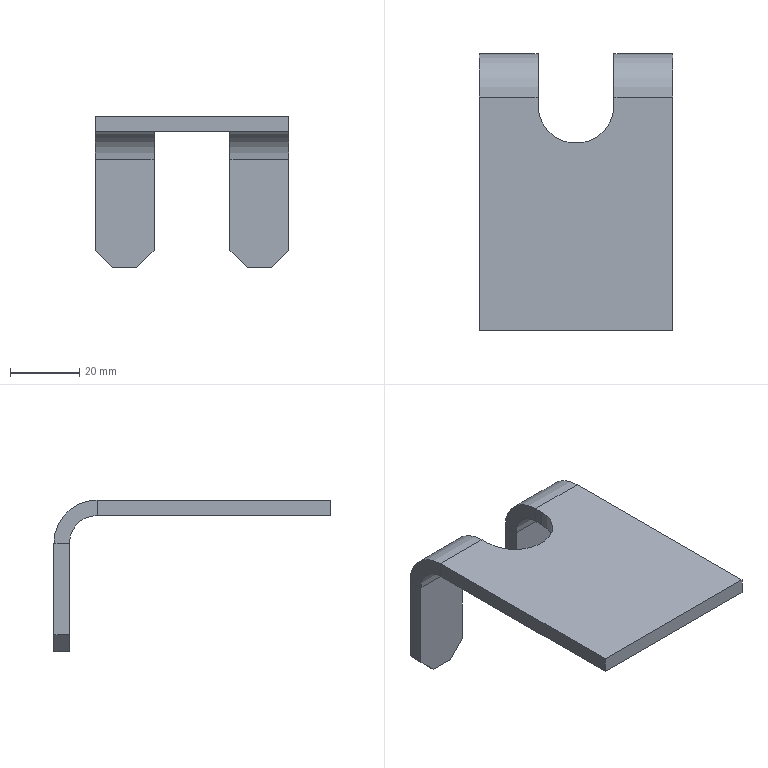Part | SolidWorks | features Chamfer 1, FlatPattern 1, ICE 1, SMBaseFlange 1, SheetMetal 1 | 1 solid | 30 faces | box 56 x 80 x 44 mm | volume 22975 mm3 | plane 25 | cylinder 5 | commonest cylinder face diameters 16 x2 25 x2 22 x1
STEP:
#1=CARTESIAN_POINT('',(39.,0.,5.));
#2=VERTEX_POINT('',#1);
#3=CARTESIAN_POINT('',(39.,0.,31.5));
#4=VERTEX_POINT('',#3);
#5=CARTESIAN_POINT('',(39.,0.,0.));
#6=DIRECTION('',(0.,0.,1.));
#7=VECTOR('',#6,1000.);
#8=LINE('',#5,#7);
#9=EDGE_CURVE('',#2,#4,#8,.T.);
#10=ORIENTED_EDGE('',*,*,#9,.F.);
#11=CARTESIAN_POINT('',(39.,-4.5,5.));
#12=VERTEX_POINT('',#11);
#13=CARTESIAN_POINT('',(39.,-4.5,5.));
#14=DIRECTION('',(0.,-1.,0.));
#15=VECTOR('',#14,1000.);
#16=LINE('',#13,#15);
#17=EDGE_CURVE('',#2,#12,#16,.T.);
#18=ORIENTED_EDGE('',*,*,#17,.T.);
#19=CARTESIAN_POINT('',(39.,-4.5,31.5));
#20=VERTEX_POINT('',#19);
#21=CARTESIAN_POINT('',(39.,-4.5,0.));
#22=DIRECTION('',(0.,0.,1.));
#23=VECTOR('',#22,1000.);
#24=LINE('',#21,#23);
#25=EDGE_CURVE('',#12,#20,#24,.T.);
#26=ORIENTED_EDGE('',*,*,#25,.T.);
#27=CARTESIAN_POINT('',(39.,-4.5,31.5));
#28=DIRECTION('',(0.,1.,0.));
#29=VECTOR('',#28,1000.);
#30=LINE('',#27,#29);
#31=EDGE_CURVE('',#20,#4,#30,.T.);
#32=ORIENTED_EDGE('',*,*,#31,.T.);
#33=EDGE_LOOP('',(#10,#18,#26,#32));
#34=FACE_OUTER_BOUND('',#33,.T.);
#35=CARTESIAN_POINT('',(39.,-14.9,0.));
#36=DIRECTION('',(1.,0.,0.));
#37=DIRECTION('',(0.,1.,0.));
#38=AXIS2_PLACEMENT_3D('',#35,#36,#37);
#39=PLANE('',#38);
#40=ADVANCED_FACE('',(#34),#39,.F.);
#41=CARTESIAN_POINT('',(39.,-14.9,44.));
#42=VERTEX_POINT('',#41);
#43=CARTESIAN_POINT('',(39.,-12.5,44.));
#44=VERTEX_POINT('',#43);
#45=CARTESIAN_POINT('',(39.,-14.9,44.));
#46=DIRECTION('',(0.,1.,0.));
#47=VECTOR('',#46,1000.);
#48=LINE('',#45,#47);
#49=EDGE_CURVE('',#42,#44,#48,.T.);
#50=ORIENTED_EDGE('',*,*,#49,.T.);
#51=CARTESIAN_POINT('',(39.,-12.5,39.5));
#52=VERTEX_POINT('',#51);
#53=CARTESIAN_POINT('',(39.,-12.5,44.));
#54=DIRECTION('',(0.,0.,-1.));
#55=VECTOR('',#54,1000.);
#56=LINE('',#53,#55);
#57=EDGE_CURVE('',#44,#52,#56,.T.);
#58=ORIENTED_EDGE('',*,*,#57,.T.);
#59=CARTESIAN_POINT('',(39.,-14.9,39.5));
#60=VERTEX_POINT('',#59);
#61=CARTESIAN_POINT('',(39.,0.,39.5));
#62=DIRECTION('',(0.,-1.,0.));
#63=VECTOR('',#62,1000.);
#64=LINE('',#61,#63);
#65=EDGE_CURVE('',#52,#60,#64,.T.);
#66=ORIENTED_EDGE('',*,*,#65,.T.);
#67=CARTESIAN_POINT('',(39.,-14.9,0.));
#68=DIRECTION('',(0.,0.,1.));
#69=VECTOR('',#68,1000.);
#70=LINE('',#67,#69);
#71=EDGE_CURVE('',#60,#42,#70,.T.);
#72=ORIENTED_EDGE('',*,*,#71,.T.);
#73=EDGE_LOOP('',(#50,#58,#66,#72));
#74=FACE_OUTER_BOUND('',#73,.T.);
#75=CARTESIAN_POINT('',(39.,-14.9,0.));
#76=DIRECTION('',(1.,0.,0.));
#77=DIRECTION('',(0.,1.,0.));
#78=AXIS2_PLACEMENT_3D('',#75,#76,#77);
#79=PLANE('',#78);
#80=ADVANCED_FACE('',(#74),#79,.F.);
#81=CARTESIAN_POINT('',(17.,-4.5,31.5));
#82=VERTEX_POINT('',#81);
#83=CARTESIAN_POINT('',(17.,-4.5,5.));
#84=VERTEX_POINT('',#83);
#85=CARTESIAN_POINT('',(17.,-4.5,0.));
#86=DIRECTION('',(0.,0.,-1.));
#87=VECTOR('',#86,1000.);
#88=LINE('',#85,#87);
#89=EDGE_CURVE('',#82,#84,#88,.T.);
#90=ORIENTED_EDGE('',*,*,#89,.T.);
#91=CARTESIAN_POINT('',(17.,0.,5.));
#92=VERTEX_POINT('',#91);
#93=CARTESIAN_POINT('',(17.,0.,5.));
#94=DIRECTION('',(0.,1.,0.));
#95=VECTOR('',#94,1000.);
#96=LINE('',#93,#95);
#97=EDGE_CURVE('',#84,#92,#96,.T.);
#98=ORIENTED_EDGE('',*,*,#97,.T.);
#99=CARTESIAN_POINT('',(17.,0.,31.5));
#100=VERTEX_POINT('',#99);
#101=CARTESIAN_POINT('',(17.,0.,0.));
#102=DIRECTION('',(0.,0.,-1.));
#103=VECTOR('',#102,1000.);
#104=LINE('',#101,#103);
#105=EDGE_CURVE('',#100,#92,#104,.T.);
#106=ORIENTED_EDGE('',*,*,#105,.F.);
#107=CARTESIAN_POINT('',(17.,0.,31.5));
#108=DIRECTION('',(0.,-1.,0.));
#109=VECTOR('',#108,1000.);
#110=LINE('',#107,#109);
#111=EDGE_CURVE('',#100,#82,#110,.T.);
#112=ORIENTED_EDGE('',*,*,#111,.T.);
#113=EDGE_LOOP('',(#90,#98,#106,#112));
#114=FACE_OUTER_BOUND('',#113,.T.);
#115=CARTESIAN_POINT('',(17.,-14.9,0.));
#116=DIRECTION('',(-1.,0.,0.));
#117=DIRECTION('',(0.,-1.,0.));
#118=AXIS2_PLACEMENT_3D('',#115,#116,#117);
#119=PLANE('',#118);
#120=ADVANCED_FACE('',(#114),#119,.F.);
#121=CARTESIAN_POINT('',(17.,-14.9,39.5));
#122=VERTEX_POINT('',#121);
#123=CARTESIAN_POINT('',(17.,-12.5,39.5));
#124=VERTEX_POINT('',#123);
#125=CARTESIAN_POINT('',(17.,0.,39.5));
#126=DIRECTION('',(0.,1.,0.));
#127=VECTOR('',#126,1000.);
#128=LINE('',#125,#127);
#129=EDGE_CURVE('',#122,#124,#128,.T.);
#130=ORIENTED_EDGE('',*,*,#129,.T.);
#131=CARTESIAN_POINT('',(17.,-12.5,44.));
#132=VERTEX_POINT('',#131);
#133=CARTESIAN_POINT('',(17.,-12.5,39.5));
#134=DIRECTION('',(0.,0.,1.));
#135=VECTOR('',#134,1000.);
#136=LINE('',#133,#135);
#137=EDGE_CURVE('',#124,#132,#136,.T.);
#138=ORIENTED_EDGE('',*,*,#137,.T.);
#139=CARTESIAN_POINT('',(17.,-14.9,44.));
#140=VERTEX_POINT('',#139);
#141=CARTESIAN_POINT('',(17.,-14.9,44.));
#142=DIRECTION('',(0.,-1.,0.));
#143=VECTOR('',#142,1000.);
#144=LINE('',#141,#143);
#145=EDGE_CURVE('',#132,#140,#144,.T.);
#146=ORIENTED_EDGE('',*,*,#145,.T.);
#147=CARTESIAN_POINT('',(17.,-14.9,0.));
#148=DIRECTION('',(0.,0.,1.));
#149=VECTOR('',#148,1000.);
#150=LINE('',#147,#149);
#151=EDGE_CURVE('',#122,#140,#150,.T.);
#152=ORIENTED_EDGE('',*,*,#151,.F.);
#153=EDGE_LOOP('',(#130,#138,#146,#152));
#154=FACE_OUTER_BOUND('',#153,.T.);
#155=CARTESIAN_POINT('',(17.,-14.9,0.));
#156=DIRECTION('',(-1.,0.,0.));
#157=DIRECTION('',(0.,-1.,0.));
#158=AXIS2_PLACEMENT_3D('',#155,#156,#157);
#159=PLANE('',#158);
#160=ADVANCED_FACE('',(#154),#159,.F.);
#161=CARTESIAN_POINT('',(17.,-12.5,31.5));
#162=DIRECTION('',(-1.,0.,0.));
#163=DIRECTION('',(0.,-1.,0.));
#164=AXIS2_PLACEMENT_3D('',#161,#162,#163);
#165=CIRCLE('',#164,8.);
#166=EDGE_CURVE('',#124,#82,#165,.T.);
#167=ORIENTED_EDGE('',*,*,#166,.F.);
#168=CARTESIAN_POINT('',(0.,-12.5,39.5));
#169=VERTEX_POINT('',#168);
#170=CARTESIAN_POINT('',(56.,-12.5,39.5));
#171=DIRECTION('',(-1.,0.,0.));
#172=VECTOR('',#171,1000.);
#173=LINE('',#170,#172);
#174=EDGE_CURVE('',#124,#169,#173,.T.);
#175=ORIENTED_EDGE('',*,*,#174,.T.);
#176=CARTESIAN_POINT('',(0.,-4.5,31.5));
#177=VERTEX_POINT('',#176);
#178=CARTESIAN_POINT('',(0.,-12.5,31.5));
#179=DIRECTION('',(1.,0.,0.));
#180=DIRECTION('',(0.,0.,-1.));
#181=AXIS2_PLACEMENT_3D('',#178,#179,#180);
#182=CIRCLE('',#181,8.);
#183=EDGE_CURVE('',#177,#169,#182,.T.);
#184=ORIENTED_EDGE('',*,*,#183,.F.);
#185=CARTESIAN_POINT('',(56.,-4.5,31.5));
#186=DIRECTION('',(-1.,0.,0.));
#187=VECTOR('',#186,1000.);
#188=LINE('',#185,#187);
#189=EDGE_CURVE('',#82,#177,#188,.T.);
#190=ORIENTED_EDGE('',*,*,#189,.F.);
#191=EDGE_LOOP('',(#167,#175,#184,#190));
#192=FACE_OUTER_BOUND('',#191,.T.);
#193=CARTESIAN_POINT('',(56.,-12.5,31.5));
#194=DIRECTION('',(-1.,0.,0.));
#195=DIRECTION('',(0.,0.,1.));
#196=AXIS2_PLACEMENT_3D('',#193,#194,#195);
#197=CYLINDRICAL_SURFACE('',#196,8.);
#198=ADVANCED_FACE('',(#192),#197,.F.);
#199=CARTESIAN_POINT('',(0.,-4.5,5.));
#200=VERTEX_POINT('',#199);
#201=CARTESIAN_POINT('',(0.,-4.5,0.));
#202=DIRECTION('',(0.,0.,1.));
#203=VECTOR('',#202,1000.);
#204=LINE('',#201,#203);
#205=EDGE_CURVE('',#200,#177,#204,.T.);
#206=ORIENTED_EDGE('',*,*,#205,.F.);
#207=CARTESIAN_POINT('',(5.,-4.5,0.));
#208=VERTEX_POINT('',#207);
#209=CARTESIAN_POINT('',(30.5,-4.5,-25.5));
#210=DIRECTION('',(0.7071,0.,-0.7071));
#211=VECTOR('',#210,1000.);
#212=LINE('',#209,#211);
#213=EDGE_CURVE('',#200,#208,#212,.T.);
#214=ORIENTED_EDGE('',*,*,#213,.T.);
#215=CARTESIAN_POINT('',(12.,-4.5,0.));
#216=VERTEX_POINT('',#215);
#217=CARTESIAN_POINT('',(56.,-4.5,0.));
#218=DIRECTION('',(-1.,0.,0.));
#219=VECTOR('',#218,1000.);
#220=LINE('',#217,#219);
#221=EDGE_CURVE('',#216,#208,#220,.T.);
#222=ORIENTED_EDGE('',*,*,#221,.F.);
#223=CARTESIAN_POINT('',(34.,-4.5,22.));
#224=DIRECTION('',(0.7071,0.,0.7071));
#225=VECTOR('',#224,1000.);
#226=LINE('',#223,#225);
#227=EDGE_CURVE('',#216,#84,#226,.T.);
#228=ORIENTED_EDGE('',*,*,#227,.T.);
#229=ORIENTED_EDGE('',*,*,#89,.F.);
#230=ORIENTED_EDGE('',*,*,#189,.T.);
#231=EDGE_LOOP('',(#206,#214,#222,#228,#229,#230));
#232=FACE_OUTER_BOUND('',#231,.T.);
#233=CARTESIAN_POINT('',(56.,-4.5,0.));
#234=DIRECTION('',(0.,-1.,0.));
#235=DIRECTION('',(0.,0.,-1.));
#236=AXIS2_PLACEMENT_3D('',#233,#234,#235);
#237=PLANE('',#236);
#238=ADVANCED_FACE('',(#232),#237,.T.);
#239=ORIENTED_EDGE('',*,*,#221,.T.);
#240=CARTESIAN_POINT('',(5.,0.,0.));
#241=VERTEX_POINT('',#240);
#242=CARTESIAN_POINT('',(5.,0.,0.));
#243=DIRECTION('',(0.,1.,0.));
#244=VECTOR('',#243,1000.);
#245=LINE('',#242,#244);
#246=EDGE_CURVE('',#208,#241,#245,.T.);
#247=ORIENTED_EDGE('',*,*,#246,.T.);
#248=CARTESIAN_POINT('',(12.,0.,0.));
#249=VERTEX_POINT('',#248);
#250=CARTESIAN_POINT('',(56.,0.,0.));
#251=DIRECTION('',(-1.,0.,0.));
#252=VECTOR('',#251,1000.);
#253=LINE('',#250,#252);
#254=EDGE_CURVE('',#249,#241,#253,.T.);
#255=ORIENTED_EDGE('',*,*,#254,.F.);
#256=CARTESIAN_POINT('',(12.,-4.5,0.));
#257=DIRECTION('',(0.,-1.,0.));
#258=VECTOR('',#257,1000.);
#259=LINE('',#256,#258);
#260=EDGE_CURVE('',#249,#216,#259,.T.);
#261=ORIENTED_EDGE('',*,*,#260,.T.);
#262=EDGE_LOOP('',(#239,#247,#255,#261));
#263=FACE_OUTER_BOUND('',#262,.T.);
#264=CARTESIAN_POINT('',(56.,0.,0.));
#265=DIRECTION('',(0.,0.,-1.));
#266=DIRECTION('',(-1.,0.,0.));
#267=AXIS2_PLACEMENT_3D('',#264,#265,#266);
#268=PLANE('',#267);
#269=ADVANCED_FACE('',(#263),#268,.T.);
#270=ORIENTED_EDGE('',*,*,#254,.T.);
#271=CARTESIAN_POINT('',(0.,0.,5.));
#272=VERTEX_POINT('',#271);
#273=CARTESIAN_POINT('',(0.,0.,5.));
#274=DIRECTION('',(-0.7071,0.,0.7071));
#275=VECTOR('',#274,1000.);
#276=LINE('',#273,#275);
#277=EDGE_CURVE('',#241,#272,#276,.T.);
#278=ORIENTED_EDGE('',*,*,#277,.T.);
#279=CARTESIAN_POINT('',(0.,0.,31.5));
#280=VERTEX_POINT('',#279);
#281=CARTESIAN_POINT('',(0.,0.,0.));
#282=DIRECTION('',(0.,0.,1.));
#283=VECTOR('',#282,1000.);
#284=LINE('',#281,#283);
#285=EDGE_CURVE('',#272,#280,#284,.T.);
#286=ORIENTED_EDGE('',*,*,#285,.T.);
#287=CARTESIAN_POINT('',(56.,0.,31.5));
#288=DIRECTION('',(-1.,0.,0.));
#289=VECTOR('',#288,1000.);
#290=LINE('',#287,#289);
#291=EDGE_CURVE('',#100,#280,#290,.T.);
#292=ORIENTED_EDGE('',*,*,#291,.F.);
#293=ORIENTED_EDGE('',*,*,#105,.T.);
#294=CARTESIAN_POINT('',(12.,0.,0.));
#295=DIRECTION('',(-0.7071,0.,-0.7071));
#296=VECTOR('',#295,1000.);
#297=LINE('',#294,#296);
#298=EDGE_CURVE('',#92,#249,#297,.T.);
#299=ORIENTED_EDGE('',*,*,#298,.T.);
#300=EDGE_LOOP('',(#270,#278,#286,#292,#293,#299));
#301=FACE_OUTER_BOUND('',#300,.T.);
#302=CARTESIAN_POINT('',(56.,0.,0.));
#303=DIRECTION('',(0.,-1.,0.));
#304=DIRECTION('',(0.,0.,-1.));
#305=AXIS2_PLACEMENT_3D('',#302,#303,#304);
#306=PLANE('',#305);
#307=ADVANCED_FACE('',(#301),#306,.F.);
#308=CARTESIAN_POINT('',(0.,-12.5,44.));
#309=VERTEX_POINT('',#308);
#310=CARTESIAN_POINT('',(56.,-12.5,44.));
#311=DIRECTION('',(-1.,0.,0.));
#312=VECTOR('',#311,1000.);
#313=LINE('',#310,#312);
#314=EDGE_CURVE('',#132,#309,#313,.T.);
#315=ORIENTED_EDGE('',*,*,#314,.F.);
#316=CARTESIAN_POINT('',(17.,-12.5,31.5));
#317=DIRECTION('',(-1.,0.,0.));
#318=DIRECTION('',(0.,-1.,0.));
#319=AXIS2_PLACEMENT_3D('',#316,#317,#318);
#320=CIRCLE('',#319,12.5);
#321=EDGE_CURVE('',#132,#100,#320,.T.);
#322=ORIENTED_EDGE('',*,*,#321,.T.);
#323=ORIENTED_EDGE('',*,*,#291,.T.);
#324=CARTESIAN_POINT('',(0.,-12.5,31.5));
#325=DIRECTION('',(1.,0.,0.));
#326=DIRECTION('',(0.,0.,1.));
#327=AXIS2_PLACEMENT_3D('',#324,#325,#326);
#328=CIRCLE('',#327,12.5);
#329=EDGE_CURVE('',#280,#309,#328,.T.);
#330=ORIENTED_EDGE('',*,*,#329,.T.);
#331=EDGE_LOOP('',(#315,#322,#323,#330));
#332=FACE_OUTER_BOUND('',#331,.T.);
#333=CARTESIAN_POINT('',(56.,-12.5,31.5));
#334=DIRECTION('',(-1.,0.,0.));
#335=DIRECTION('',(0.,0.,1.));
#336=AXIS2_PLACEMENT_3D('',#333,#334,#335);
#337=CYLINDRICAL_SURFACE('',#336,12.5);
#338=ADVANCED_FACE('',(#332),#337,.T.);
#339=CARTESIAN_POINT('',(56.,0.,31.5));
#340=VERTEX_POINT('',#339);
#341=CARTESIAN_POINT('',(56.,-4.5,31.5));
#342=VERTEX_POINT('',#341);
#343=CARTESIAN_POINT('',(56.,0.,31.5));
#344=DIRECTION('',(0.,-1.,0.));
#345=VECTOR('',#344,1000.);
#346=LINE('',#343,#345);
#347=EDGE_CURVE('',#340,#342,#346,.T.);
#348=ORIENTED_EDGE('',*,*,#347,.F.);
#349=CARTESIAN_POINT('',(56.,-12.5,44.));
#350=VERTEX_POINT('',#349);
#351=CARTESIAN_POINT('',(56.,-12.5,31.5));
#352=DIRECTION('',(1.,0.,0.));
#353=DIRECTION('',(0.,0.,1.));
#354=AXIS2_PLACEMENT_3D('',#351,#352,#353);
#355=CIRCLE('',#354,12.5);
#356=EDGE_CURVE('',#340,#350,#355,.T.);
#357=ORIENTED_EDGE('',*,*,#356,.T.);
#358=CARTESIAN_POINT('',(56.,-12.5,39.5));
#359=VERTEX_POINT('',#358);
#360=CARTESIAN_POINT('',(56.,-12.5,39.5));
#361=DIRECTION('',(0.,0.,1.));
#362=VECTOR('',#361,1000.);
#363=LINE('',#360,#362);
#364=EDGE_CURVE('',#359,#350,#363,.T.);
#365=ORIENTED_EDGE('',*,*,#364,.F.);
#366=CARTESIAN_POINT('',(56.,-12.5,31.5));
#367=DIRECTION('',(1.,0.,0.));
#368=DIRECTION('',(0.,0.,-1.));
#369=AXIS2_PLACEMENT_3D('',#366,#367,#368);
#370=CIRCLE('',#369,8.);
#371=EDGE_CURVE('',#342,#359,#370,.T.);
#372=ORIENTED_EDGE('',*,*,#371,.F.);
#373=EDGE_LOOP('',(#348,#357,#365,#372));
#374=FACE_OUTER_BOUND('',#373,.T.);
#375=CARTESIAN_POINT('',(56.,0.,31.5));
#376=DIRECTION('',(1.,0.,0.));
#377=DIRECTION('',(0.,0.,-1.));
#378=AXIS2_PLACEMENT_3D('',#375,#376,#377);
#379=PLANE('',#378);
#380=ADVANCED_FACE('',(#374),#379,.T.);
#381=CARTESIAN_POINT('',(56.,-4.5,5.));
#382=VERTEX_POINT('',#381);
#383=CARTESIAN_POINT('',(56.,-4.5,0.));
#384=DIRECTION('',(0.,0.,1.));
#385=VECTOR('',#384,1000.);
#386=LINE('',#383,#385);
#387=EDGE_CURVE('',#382,#342,#386,.T.);
#388=ORIENTED_EDGE('',*,*,#387,.F.);
#389=CARTESIAN_POINT('',(56.,0.,5.));
#390=VERTEX_POINT('',#389);
#391=CARTESIAN_POINT('',(56.,-12.5,5.));
#392=DIRECTION('',(0.,1.,0.));
#393=VECTOR('',#392,1000.);
#394=LINE('',#391,#393);
#395=EDGE_CURVE('',#382,#390,#394,.T.);
#396=ORIENTED_EDGE('',*,*,#395,.T.);
#397=CARTESIAN_POINT('',(56.,0.,0.));
#398=DIRECTION('',(0.,0.,1.));
#399=VECTOR('',#398,1000.);
#400=LINE('',#397,#399);
#401=EDGE_CURVE('',#390,#340,#400,.T.);
#402=ORIENTED_EDGE('',*,*,#401,.T.);
#403=ORIENTED_EDGE('',*,*,#347,.T.);
#404=EDGE_LOOP('',(#388,#396,#402,#403));
#405=FACE_OUTER_BOUND('',#404,.T.);
#406=CARTESIAN_POINT('',(56.,-12.5,39.5));
#407=DIRECTION('',(1.,0.,0.));
#408=DIRECTION('',(0.,0.,-1.));
#409=AXIS2_PLACEMENT_3D('',#406,#407,#408);
#410=PLANE('',#409);
#411=ADVANCED_FACE('',(#405),#410,.T.);
#412=CARTESIAN_POINT('',(0.,-12.5,44.));
#413=DIRECTION('',(0.,0.,-1.));
#414=VECTOR('',#413,1000.);
#415=LINE('',#412,#414);
#416=EDGE_CURVE('',#309,#169,#415,.T.);
#417=ORIENTED_EDGE('',*,*,#416,.F.);
#418=ORIENTED_EDGE('',*,*,#329,.F.);
#419=CARTESIAN_POINT('',(0.,-4.5,31.5));
#420=DIRECTION('',(0.,1.,0.));
#421=VECTOR('',#420,1000.);
#422=LINE('',#419,#421);
#423=EDGE_CURVE('',#177,#280,#422,.T.);
#424=ORIENTED_EDGE('',*,*,#423,.F.);
#425=ORIENTED_EDGE('',*,*,#183,.T.);
#426=EDGE_LOOP('',(#417,#418,#424,#425));
#427=FACE_OUTER_BOUND('',#426,.T.);
#428=CARTESIAN_POINT('',(0.,-12.5,44.));
#429=DIRECTION('',(-1.,0.,0.));
#430=DIRECTION('',(0.,0.,1.));
#431=AXIS2_PLACEMENT_3D('',#428,#429,#430);
#432=PLANE('',#431);
#433=ADVANCED_FACE('',(#427),#432,.T.);
#434=CARTESIAN_POINT('',(0.,-80.,44.));
#435=VERTEX_POINT('',#434);
#436=CARTESIAN_POINT('',(0.,0.,44.));
#437=DIRECTION('',(0.,-1.,0.));
#438=VECTOR('',#437,1000.);
#439=LINE('',#436,#438);
#440=EDGE_CURVE('',#309,#435,#439,.T.);
#441=ORIENTED_EDGE('',*,*,#440,.F.);
#442=ORIENTED_EDGE('',*,*,#416,.T.);
#443=CARTESIAN_POINT('',(0.,-80.,39.5));
#444=VERTEX_POINT('',#443);
#445=CARTESIAN_POINT('',(0.,0.,39.5));
#446=DIRECTION('',(0.,-1.,0.));
#447=VECTOR('',#446,1000.);
#448=LINE('',#445,#447);
#449=EDGE_CURVE('',#169,#444,#448,.T.);
#450=ORIENTED_EDGE('',*,*,#449,.T.);
#451=CARTESIAN_POINT('',(0.,-80.,39.5));
#452=DIRECTION('',(0.,0.,1.));
#453=VECTOR('',#452,1000.);
#454=LINE('',#451,#453);
#455=EDGE_CURVE('',#444,#435,#454,.T.);
#456=ORIENTED_EDGE('',*,*,#455,.T.);
#457=EDGE_LOOP('',(#441,#442,#450,#456));
#458=FACE_OUTER_BOUND('',#457,.T.);
#459=CARTESIAN_POINT('',(0.,-4.5,31.5));
#460=DIRECTION('',(-1.,0.,0.));
#461=DIRECTION('',(0.,0.,1.));
#462=AXIS2_PLACEMENT_3D('',#459,#460,#461);
#463=PLANE('',#462);
#464=ADVANCED_FACE('',(#458),#463,.T.);
#465=CARTESIAN_POINT('',(28.,-14.9,44.));
#466=DIRECTION('',(0.,0.,1.));
#467=DIRECTION('',(1.,0.,0.));
#468=AXIS2_PLACEMENT_3D('',#465,#466,#467);
#469=CIRCLE('',#468,11.);
#470=EDGE_CURVE('',#140,#42,#469,.T.);
#471=ORIENTED_EDGE('',*,*,#470,.F.);
#472=ORIENTED_EDGE('',*,*,#145,.F.);
#473=ORIENTED_EDGE('',*,*,#314,.T.);
#474=ORIENTED_EDGE('',*,*,#440,.T.);
#475=CARTESIAN_POINT('',(56.,-80.,44.));
#476=VERTEX_POINT('',#475);
#477=CARTESIAN_POINT('',(56.,-80.,44.));
#478=DIRECTION('',(-1.,0.,0.));
#479=VECTOR('',#478,1000.);
#480=LINE('',#477,#479);
#481=EDGE_CURVE('',#476,#435,#480,.T.);
#482=ORIENTED_EDGE('',*,*,#481,.F.);
#483=CARTESIAN_POINT('',(56.,0.,44.));
#484=DIRECTION('',(0.,-1.,0.));
#485=VECTOR('',#484,1000.);
#486=LINE('',#483,#485);
#487=EDGE_CURVE('',#350,#476,#486,.T.);
#488=ORIENTED_EDGE('',*,*,#487,.F.);
#489=CARTESIAN_POINT('',(56.,-12.5,44.));
#490=DIRECTION('',(-1.,0.,0.));
#491=VECTOR('',#490,1000.);
#492=LINE('',#489,#491);
#493=EDGE_CURVE('',#350,#44,#492,.T.);
#494=ORIENTED_EDGE('',*,*,#493,.T.);
#495=ORIENTED_EDGE('',*,*,#49,.F.);
#496=EDGE_LOOP('',(#471,#472,#473,#474,#482,#488,#494,#495));
#497=FACE_OUTER_BOUND('',#496,.T.);
#498=CARTESIAN_POINT('',(56.,0.,44.));
#499=DIRECTION('',(0.,0.,-1.));
#500=DIRECTION('',(0.,1.,0.));
#501=AXIS2_PLACEMENT_3D('',#498,#499,#500);
#502=PLANE('',#501);
#503=ADVANCED_FACE('',(#497),#502,.F.);
#504=ORIENTED_EDGE('',*,*,#455,.F.);
#505=CARTESIAN_POINT('',(56.,-80.,39.5));
#506=VERTEX_POINT('',#505);
#507=CARTESIAN_POINT('',(56.,-80.,39.5));
#508=DIRECTION('',(-1.,0.,0.));
#509=VECTOR('',#508,1000.);
#510=LINE('',#507,#509);
#511=EDGE_CURVE('',#506,#444,#510,.T.);
#512=ORIENTED_EDGE('',*,*,#511,.F.);
#513=CARTESIAN_POINT('',(56.,-80.,39.5));
#514=DIRECTION('',(0.,0.,1.));
#515=VECTOR('',#514,1000.);
#516=LINE('',#513,#515);
#517=EDGE_CURVE('',#506,#476,#516,.T.);
#518=ORIENTED_EDGE('',*,*,#517,.T.);
#519=ORIENTED_EDGE('',*,*,#481,.T.);
#520=EDGE_LOOP('',(#504,#512,#518,#519));
#521=FACE_OUTER_BOUND('',#520,.T.);
#522=CARTESIAN_POINT('',(56.,-80.,39.5));
#523=DIRECTION('',(0.,-1.,0.));
#524=DIRECTION('',(0.,0.,-1.));
#525=AXIS2_PLACEMENT_3D('',#522,#523,#524);
#526=PLANE('',#525);
#527=ADVANCED_FACE('',(#521),#526,.T.);
#528=ORIENTED_EDGE('',*,*,#129,.F.);
#529=CARTESIAN_POINT('',(28.,-14.9,39.5));
#530=DIRECTION('',(0.,0.,-1.));
#531=DIRECTION('',(0.,1.,0.));
#532=AXIS2_PLACEMENT_3D('',#529,#530,#531);
#533=CIRCLE('',#532,11.);
#534=EDGE_CURVE('',#60,#122,#533,.T.);
#535=ORIENTED_EDGE('',*,*,#534,.F.);
#536=ORIENTED_EDGE('',*,*,#65,.F.);
#537=CARTESIAN_POINT('',(56.,-12.5,39.5));
#538=DIRECTION('',(-1.,0.,0.));
#539=VECTOR('',#538,1000.);
#540=LINE('',#537,#539);
#541=EDGE_CURVE('',#359,#52,#540,.T.);
#542=ORIENTED_EDGE('',*,*,#541,.F.);
#543=CARTESIAN_POINT('',(56.,0.,39.5));
#544=DIRECTION('',(0.,-1.,0.));
#545=VECTOR('',#544,1000.);
#546=LINE('',#543,#545);
#547=EDGE_CURVE('',#359,#506,#546,.T.);
#548=ORIENTED_EDGE('',*,*,#547,.T.);
#549=ORIENTED_EDGE('',*,*,#511,.T.);
#550=ORIENTED_EDGE('',*,*,#449,.F.);
#551=ORIENTED_EDGE('',*,*,#174,.F.);
#552=EDGE_LOOP('',(#528,#535,#536,#542,#548,#549,#550,#551));
#553=FACE_OUTER_BOUND('',#552,.T.);
#554=CARTESIAN_POINT('',(56.,0.,39.5));
#555=DIRECTION('',(0.,0.,-1.));
#556=DIRECTION('',(0.,1.,0.));
#557=AXIS2_PLACEMENT_3D('',#554,#555,#556);
#558=PLANE('',#557);
#559=ADVANCED_FACE('',(#553),#558,.T.);
#560=CARTESIAN_POINT('',(39.,-12.5,31.5));
#561=DIRECTION('',(1.,0.,0.));
#562=DIRECTION('',(0.,1.,0.));
#563=AXIS2_PLACEMENT_3D('',#560,#561,#562);
#564=CIRCLE('',#563,8.);
#565=EDGE_CURVE('',#20,#52,#564,.T.);
#566=ORIENTED_EDGE('',*,*,#565,.F.);
#567=CARTESIAN_POINT('',(56.,-4.5,31.5));
#568=DIRECTION('',(-1.,0.,0.));
#569=VECTOR('',#568,1000.);
#570=LINE('',#567,#569);
#571=EDGE_CURVE('',#342,#20,#570,.T.);
#572=ORIENTED_EDGE('',*,*,#571,.F.);
#573=ORIENTED_EDGE('',*,*,#371,.T.);
#574=ORIENTED_EDGE('',*,*,#541,.T.);
#575=EDGE_LOOP('',(#566,#572,#573,#574));
#576=FACE_OUTER_BOUND('',#575,.T.);
#577=CARTESIAN_POINT('',(56.,-12.5,31.5));
#578=DIRECTION('',(-1.,0.,0.));
#579=DIRECTION('',(0.,0.,1.));
#580=AXIS2_PLACEMENT_3D('',#577,#578,#579);
#581=CYLINDRICAL_SURFACE('',#580,8.);
#582=ADVANCED_FACE('',(#576),#581,.F.);
#583=ORIENTED_EDGE('',*,*,#25,.F.);
#584=CARTESIAN_POINT('',(44.,-4.5,0.));
#585=VERTEX_POINT('',#584);
#586=CARTESIAN_POINT('',(50.,-4.5,-6.));
#587=DIRECTION('',(0.7071,0.,-0.7071));
#588=VECTOR('',#587,1000.);
#589=LINE('',#586,#588);
#590=EDGE_CURVE('',#12,#585,#589,.T.);
#591=ORIENTED_EDGE('',*,*,#590,.T.);
#592=CARTESIAN_POINT('',(51.,-4.5,0.));
#593=VERTEX_POINT('',#592);
#594=CARTESIAN_POINT('',(56.,-4.5,0.));
#595=DIRECTION('',(-1.,0.,0.));
#596=VECTOR('',#595,1000.);
#597=LINE('',#594,#596);
#598=EDGE_CURVE('',#593,#585,#597,.T.);
#599=ORIENTED_EDGE('',*,*,#598,.F.);
#600=CARTESIAN_POINT('',(53.5,-4.5,2.5));
#601=DIRECTION('',(0.7071,0.,0.7071));
#602=VECTOR('',#601,1000.);
#603=LINE('',#600,#602);
#604=EDGE_CURVE('',#593,#382,#603,.T.);
#605=ORIENTED_EDGE('',*,*,#604,.T.);
#606=ORIENTED_EDGE('',*,*,#387,.T.);
#607=ORIENTED_EDGE('',*,*,#571,.T.);
#608=EDGE_LOOP('',(#583,#591,#599,#605,#606,#607));
#609=FACE_OUTER_BOUND('',#608,.T.);
#610=CARTESIAN_POINT('',(56.,-4.5,0.));
#611=DIRECTION('',(0.,-1.,0.));
#612=DIRECTION('',(0.,0.,-1.));
#613=AXIS2_PLACEMENT_3D('',#610,#611,#612);
#614=PLANE('',#613);
#615=ADVANCED_FACE('',(#609),#614,.T.);
#616=ORIENTED_EDGE('',*,*,#598,.T.);
#617=CARTESIAN_POINT('',(44.,0.,0.));
#618=VERTEX_POINT('',#617);
#619=CARTESIAN_POINT('',(44.,0.,0.));
#620=DIRECTION('',(0.,1.,0.));
#621=VECTOR('',#620,1000.);
#622=LINE('',#619,#621);
#623=EDGE_CURVE('',#585,#618,#622,.T.);
#624=ORIENTED_EDGE('',*,*,#623,.T.);
#625=CARTESIAN_POINT('',(51.,0.,0.));
#626=VERTEX_POINT('',#625);
#627=CARTESIAN_POINT('',(56.,0.,0.));
#628=DIRECTION('',(-1.,0.,0.));
#629=VECTOR('',#628,1000.);
#630=LINE('',#627,#629);
#631=EDGE_CURVE('',#626,#618,#630,.T.);
#632=ORIENTED_EDGE('',*,*,#631,.F.);
#633=CARTESIAN_POINT('',(51.,0.,0.));
#634=DIRECTION('',(0.,-1.,0.));
#635=VECTOR('',#634,1000.);
#636=LINE('',#633,#635);
#637=EDGE_CURVE('',#626,#593,#636,.T.);
#638=ORIENTED_EDGE('',*,*,#637,.T.);
#639=EDGE_LOOP('',(#616,#624,#632,#638));
#640=FACE_OUTER_BOUND('',#639,.T.);
#641=CARTESIAN_POINT('',(56.,0.,0.));
#642=DIRECTION('',(0.,0.,-1.));
#643=DIRECTION('',(-1.,0.,0.));
#644=AXIS2_PLACEMENT_3D('',#641,#642,#643);
#645=PLANE('',#644);
#646=ADVANCED_FACE('',(#640),#645,.T.);
#647=ORIENTED_EDGE('',*,*,#631,.T.);
#648=CARTESIAN_POINT('',(44.,0.,0.));
#649=DIRECTION('',(-0.7071,0.,0.7071));
#650=VECTOR('',#649,1000.);
#651=LINE('',#648,#650);
#652=EDGE_CURVE('',#618,#2,#651,.T.);
#653=ORIENTED_EDGE('',*,*,#652,.T.);
#654=ORIENTED_EDGE('',*,*,#9,.T.);
#655=CARTESIAN_POINT('',(56.,0.,31.5));
#656=DIRECTION('',(-1.,0.,0.));
#657=VECTOR('',#656,1000.);
#658=LINE('',#655,#657);
#659=EDGE_CURVE('',#340,#4,#658,.T.);
#660=ORIENTED_EDGE('',*,*,#659,.F.);
#661=ORIENTED_EDGE('',*,*,#401,.F.);
#662=CARTESIAN_POINT('',(51.,0.,0.));
#663=DIRECTION('',(-0.7071,0.,-0.7071));
#664=VECTOR('',#663,1000.);
#665=LINE('',#662,#664);
#666=EDGE_CURVE('',#390,#626,#665,.T.);
#667=ORIENTED_EDGE('',*,*,#666,.T.);
#668=EDGE_LOOP('',(#647,#653,#654,#660,#661,#667));
#669=FACE_OUTER_BOUND('',#668,.T.);
#670=CARTESIAN_POINT('',(56.,0.,0.));
#671=DIRECTION('',(0.,-1.,0.));
#672=DIRECTION('',(0.,0.,-1.));
#673=AXIS2_PLACEMENT_3D('',#670,#671,#672);
#674=PLANE('',#673);
#675=ADVANCED_FACE('',(#669),#674,.F.);
#676=ORIENTED_EDGE('',*,*,#659,.T.);
#677=CARTESIAN_POINT('',(39.,-12.5,31.5));
#678=DIRECTION('',(1.,0.,0.));
#679=DIRECTION('',(0.,1.,0.));
#680=AXIS2_PLACEMENT_3D('',#677,#678,#679);
#681=CIRCLE('',#680,12.5);
#682=EDGE_CURVE('',#4,#44,#681,.T.);
#683=ORIENTED_EDGE('',*,*,#682,.T.);
#684=ORIENTED_EDGE('',*,*,#493,.F.);
#685=ORIENTED_EDGE('',*,*,#356,.F.);
#686=EDGE_LOOP('',(#676,#683,#684,#685));
#687=FACE_OUTER_BOUND('',#686,.T.);
#688=CARTESIAN_POINT('',(56.,-12.5,31.5));
#689=DIRECTION('',(-1.,0.,0.));
#690=DIRECTION('',(0.,0.,1.));
#691=AXIS2_PLACEMENT_3D('',#688,#689,#690);
#692=CYLINDRICAL_SURFACE('',#691,12.5);
#693=ADVANCED_FACE('',(#687),#692,.T.);
#694=ORIENTED_EDGE('',*,*,#487,.T.);
#695=ORIENTED_EDGE('',*,*,#517,.F.);
#696=ORIENTED_EDGE('',*,*,#547,.F.);
#697=ORIENTED_EDGE('',*,*,#364,.T.);
#698=EDGE_LOOP('',(#694,#695,#696,#697));
#699=FACE_OUTER_BOUND('',#698,.T.);
#700=CARTESIAN_POINT('',(56.,-12.5,31.5));
#701=DIRECTION('',(1.,0.,0.));
#702=DIRECTION('',(0.,0.,-1.));
#703=AXIS2_PLACEMENT_3D('',#700,#701,#702);
#704=PLANE('',#703);
#705=ADVANCED_FACE('',(#699),#704,.T.);
#706=ORIENTED_EDGE('',*,*,#285,.F.);
#707=CARTESIAN_POINT('',(0.,-4.5,5.));
#708=DIRECTION('',(0.,-1.,0.));
#709=VECTOR('',#708,1000.);
#710=LINE('',#707,#709);
#711=EDGE_CURVE('',#272,#200,#710,.T.);
#712=ORIENTED_EDGE('',*,*,#711,.T.);
#713=ORIENTED_EDGE('',*,*,#205,.T.);
#714=ORIENTED_EDGE('',*,*,#423,.T.);
#715=EDGE_LOOP('',(#706,#712,#713,#714));
#716=FACE_OUTER_BOUND('',#715,.T.);
#717=CARTESIAN_POINT('',(0.,-12.5,31.5));
#718=DIRECTION('',(1.,0.,0.));
#719=DIRECTION('',(0.,0.,-1.));
#720=AXIS2_PLACEMENT_3D('',#717,#718,#719);
#721=PLANE('',#720);
#722=ADVANCED_FACE('',(#716),#721,.F.);
#723=ORIENTED_EDGE('',*,*,#111,.F.);
#724=ORIENTED_EDGE('',*,*,#321,.F.);
#725=ORIENTED_EDGE('',*,*,#137,.F.);
#726=ORIENTED_EDGE('',*,*,#166,.T.);
#727=EDGE_LOOP('',(#723,#724,#725,#726));
#728=FACE_OUTER_BOUND('',#727,.T.);
#729=CARTESIAN_POINT('',(17.,-14.9,0.));
#730=DIRECTION('',(-1.,0.,0.));
#731=DIRECTION('',(0.,-1.,0.));
#732=AXIS2_PLACEMENT_3D('',#729,#730,#731);
#733=PLANE('',#732);
#734=ADVANCED_FACE('',(#728),#733,.F.);
#735=ORIENTED_EDGE('',*,*,#31,.F.);
#736=ORIENTED_EDGE('',*,*,#565,.T.);
#737=ORIENTED_EDGE('',*,*,#57,.F.);
#738=ORIENTED_EDGE('',*,*,#682,.F.);
#739=EDGE_LOOP('',(#735,#736,#737,#738));
#740=FACE_OUTER_BOUND('',#739,.T.);
#741=CARTESIAN_POINT('',(39.,-14.9,0.));
#742=DIRECTION('',(1.,0.,0.));
#743=DIRECTION('',(0.,1.,0.));
#744=AXIS2_PLACEMENT_3D('',#741,#742,#743);
#745=PLANE('',#744);
#746=ADVANCED_FACE('',(#740),#745,.F.);
#747=ORIENTED_EDGE('',*,*,#534,.T.);
#748=ORIENTED_EDGE('',*,*,#151,.T.);
#749=ORIENTED_EDGE('',*,*,#470,.T.);
#750=ORIENTED_EDGE('',*,*,#71,.F.);
#751=EDGE_LOOP('',(#747,#748,#749,#750));
#752=FACE_OUTER_BOUND('',#751,.T.);
#753=CARTESIAN_POINT('',(28.,-14.9,0.));
#754=DIRECTION('',(0.,0.,1.));
#755=DIRECTION('',(1.,0.,0.));
#756=AXIS2_PLACEMENT_3D('',#753,#754,#755);
#757=CYLINDRICAL_SURFACE('',#756,11.);
#758=ADVANCED_FACE('',(#752),#757,.F.);
#759=ORIENTED_EDGE('',*,*,#277,.F.);
#760=ORIENTED_EDGE('',*,*,#246,.F.);
#761=ORIENTED_EDGE('',*,*,#213,.F.);
#762=ORIENTED_EDGE('',*,*,#711,.F.);
#763=EDGE_LOOP('',(#759,#760,#761,#762));
#764=FACE_OUTER_BOUND('',#763,.T.);
#765=CARTESIAN_POINT('',(0.,-12.5,5.));
#766=DIRECTION('',(-0.7071,0.,-0.7071));
#767=DIRECTION('',(0.,1.,0.));
#768=AXIS2_PLACEMENT_3D('',#765,#766,#767);
#769=PLANE('',#768);
#770=ADVANCED_FACE('',(#764),#769,.T.);
#771=ORIENTED_EDGE('',*,*,#298,.F.);
#772=ORIENTED_EDGE('',*,*,#97,.F.);
#773=ORIENTED_EDGE('',*,*,#227,.F.);
#774=ORIENTED_EDGE('',*,*,#260,.F.);
#775=EDGE_LOOP('',(#771,#772,#773,#774));
#776=FACE_OUTER_BOUND('',#775,.T.);
#777=CARTESIAN_POINT('',(12.,0.,0.));
#778=DIRECTION('',(0.7071,0.,-0.7071));
#779=DIRECTION('',(0.,1.,0.));
#780=AXIS2_PLACEMENT_3D('',#777,#778,#779);
#781=PLANE('',#780);
#782=ADVANCED_FACE('',(#776),#781,.T.);
#783=ORIENTED_EDGE('',*,*,#590,.F.);
#784=ORIENTED_EDGE('',*,*,#17,.F.);
#785=ORIENTED_EDGE('',*,*,#652,.F.);
#786=ORIENTED_EDGE('',*,*,#623,.F.);
#787=EDGE_LOOP('',(#783,#784,#785,#786));
#788=FACE_OUTER_BOUND('',#787,.T.);
#789=CARTESIAN_POINT('',(44.,0.,0.));
#790=DIRECTION('',(-0.7071,0.,-0.7071));
#791=DIRECTION('',(0.,-1.,0.));
#792=AXIS2_PLACEMENT_3D('',#789,#790,#791);
#793=PLANE('',#792);
#794=ADVANCED_FACE('',(#788),#793,.T.);
#795=ORIENTED_EDGE('',*,*,#666,.F.);
#796=ORIENTED_EDGE('',*,*,#395,.F.);
#797=ORIENTED_EDGE('',*,*,#604,.F.);
#798=ORIENTED_EDGE('',*,*,#637,.F.);
#799=EDGE_LOOP('',(#795,#796,#797,#798));
#800=FACE_OUTER_BOUND('',#799,.T.);
#801=CARTESIAN_POINT('',(51.,0.,0.));
#802=DIRECTION('',(-0.7071,0.,0.7071));
#803=DIRECTION('',(0.,-1.,0.));
#804=AXIS2_PLACEMENT_3D('',#801,#802,#803);
#805=PLANE('',#804);
#806=ADVANCED_FACE('',(#800),#805,.F.);
#807=CLOSED_SHELL('',(#40,#80,#120,#160,#198,#238,#269,#307,#338,#380,#411,#433,#464,#503,#527,#559,#582,#615,#646,#675,#693,#705,#722,#734,#746,#758,#770,#782,#794,#806));
#808=MANIFOLD_SOLID_BREP('',#807);
#809=CARTESIAN_POINT('',(0.,0.,0.));
#810=DIRECTION('',(0.,0.,1.));
#811=DIRECTION('',(1.,0.,0.));
#812=AXIS2_PLACEMENT_3D('',#809,#810,#811);
#813=(LENGTH_UNIT()NAMED_UNIT(*)SI_UNIT(.MILLI.,.METRE.));
#814=UNCERTAINTY_MEASURE_WITH_UNIT(LENGTH_MEASURE(0.00001),#813,'','');
#815=(NAMED_UNIT(*)PLANE_ANGLE_UNIT()SI_UNIT($,.RADIAN.));
#816=(NAMED_UNIT(*)SI_UNIT($,.STERADIAN.)SOLID_ANGLE_UNIT());
#817=(GEOMETRIC_REPRESENTATION_CONTEXT(3)GLOBAL_UNCERTAINTY_ASSIGNED_CONTEXT((#814))GLOBAL_UNIT_ASSIGNED_CONTEXT((#813,#815,#816))REPRESENTATION_CONTEXT('',''));
#818=ADVANCED_BREP_SHAPE_REPRESENTATION('',(#808,#812),#817);